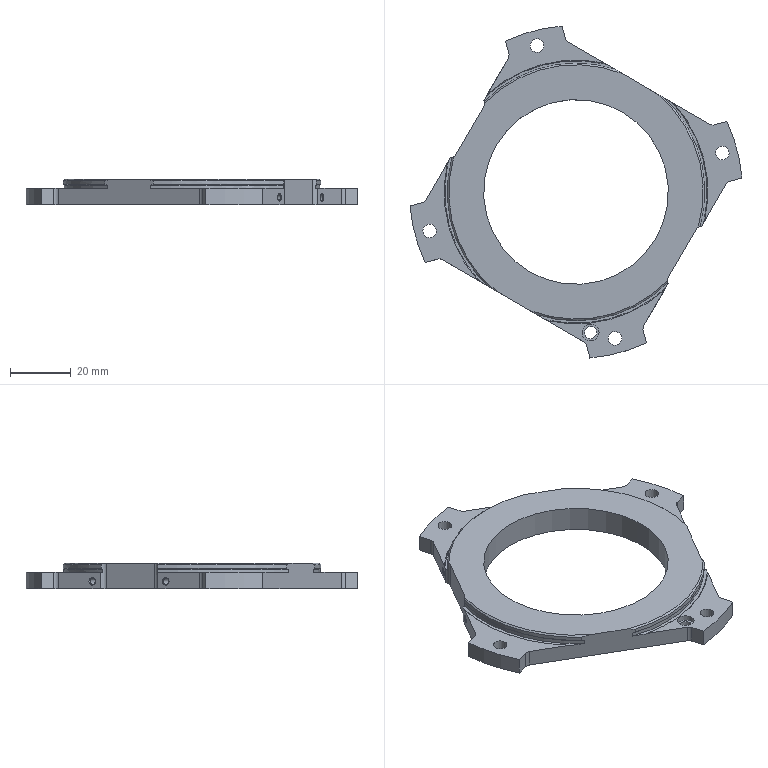Part | STEP file | 1 solid | 106 faces | box 109.615 x 109.615 x 8.5 mm | volume 28096 mm3 | cylinder 43 | plane 39 | cone 24 | commonest cylinder face diameters 4 x21 2.05 x4 4.5 x4 84.6 x4 85 x4 110 x4